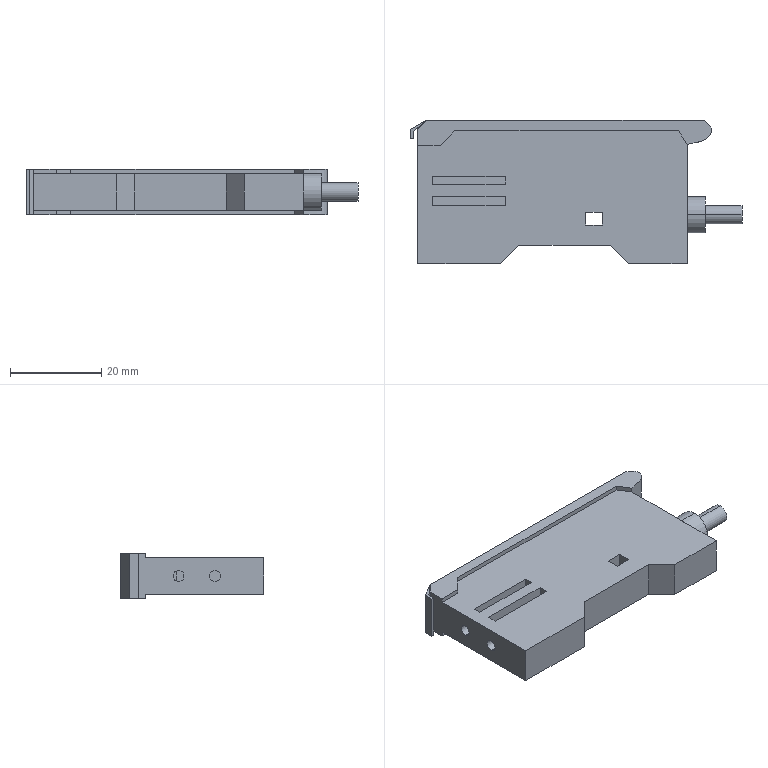Part | STEP file | E32-ZD12 | 2 solids | 58 faces | box 72.685 x 31.5 x 10 mm | volume 14433 mm3 | plane 48 | cylinder 8 | spline 2 | commonest cylinder face diameters 2.4 x4 4 x2 8 x2